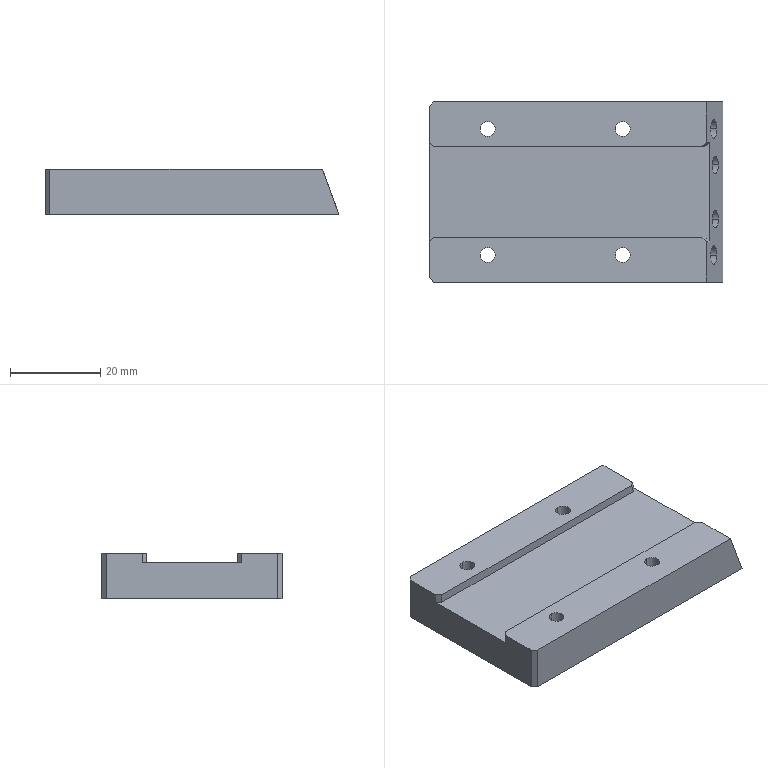Part | NX | 1 solid | 38 faces | box 65.2 x 40 x 10 mm | volume 22132 mm3 | plane 18 | cylinder 16 | cone 4 | commonest cylinder face diameters 3.3 x8 4 x4 4.2 x4
STEP:
#1=CARTESIAN_POINT('',(25.507,-6.,-5.132));
#2=VERTEX_POINT('',#1);
#3=CARTESIAN_POINT('',(26.875,-6.,-8.891));
#4=VERTEX_POINT('',#3);
#5=CARTESIAN_POINT('',(26.191,-6.,-7.012));
#6=DIRECTION('',(0.9397,0.,0.342));
#7=DIRECTION('',(0.342,0.,-0.9397));
#8=AXIS2_PLACEMENT_3D('',#5,#6,#7);
#9=CIRCLE('',#8,2.);
#10=EDGE_CURVE('',#2,#4,#9,.T.);
#11=ORIENTED_EDGE('',*,*,#10,.F.);
#12=CARTESIAN_POINT('',(30.206,-6.,-3.422));
#13=VERTEX_POINT('',#12);
#14=CARTESIAN_POINT('',(25.507,-6.,-5.132));
#15=DIRECTION('',(0.9397,0.,0.342));
#16=VECTOR('',#15,1000.);
#17=LINE('',#14,#16);
#18=EDGE_CURVE('',#2,#13,#17,.T.);
#19=ORIENTED_EDGE('',*,*,#18,.T.);
#20=CARTESIAN_POINT('',(31.574,-6.,-7.181));
#21=VERTEX_POINT('',#20);
#22=CARTESIAN_POINT('',(30.89,-6.,-5.302));
#23=DIRECTION('',(0.9397,0.,0.342));
#24=DIRECTION('',(0.342,0.,-0.9397));
#25=AXIS2_PLACEMENT_3D('',#22,#23,#24);
#26=CIRCLE('',#25,2.);
#27=EDGE_CURVE('',#13,#21,#26,.T.);
#28=ORIENTED_EDGE('',*,*,#27,.T.);
#29=CARTESIAN_POINT('',(26.875,-6.,-8.891));
#30=DIRECTION('',(0.9397,0.,0.342));
#31=VECTOR('',#30,1000.);
#32=LINE('',#29,#31);
#33=EDGE_CURVE('',#4,#21,#32,.T.);
#34=ORIENTED_EDGE('',*,*,#33,.F.);
#35=EDGE_LOOP('',(#11,#19,#28,#34));
#36=FACE_BOUND('',#35,.T.);
#37=CARTESIAN_POINT('',(26.191,-6.,-7.012));
#38=DIRECTION('',(0.9397,0.,0.342));
#39=DIRECTION('',(-0.342,0.,0.9397));
#40=AXIS2_PLACEMENT_3D('',#37,#38,#39);
#41=CYLINDRICAL_SURFACE('',#40,2.);
#42=ADVANCED_FACE('',(#36),#41,.F.);
#43=CARTESIAN_POINT('',(25.507,6.,-5.132));
#44=VERTEX_POINT('',#43);
#45=CARTESIAN_POINT('',(26.875,6.,-8.891));
#46=VERTEX_POINT('',#45);
#47=CARTESIAN_POINT('',(26.191,6.,-7.012));
#48=DIRECTION('',(0.9397,0.,0.342));
#49=DIRECTION('',(0.342,0.,-0.9397));
#50=AXIS2_PLACEMENT_3D('',#47,#48,#49);
#51=CIRCLE('',#50,2.);
#52=EDGE_CURVE('',#44,#46,#51,.T.);
#53=ORIENTED_EDGE('',*,*,#52,.F.);
#54=CARTESIAN_POINT('',(30.206,6.,-3.422));
#55=VERTEX_POINT('',#54);
#56=CARTESIAN_POINT('',(25.507,6.,-5.132));
#57=DIRECTION('',(0.9397,0.,0.342));
#58=VECTOR('',#57,1000.);
#59=LINE('',#56,#58);
#60=EDGE_CURVE('',#44,#55,#59,.T.);
#61=ORIENTED_EDGE('',*,*,#60,.T.);
#62=CARTESIAN_POINT('',(31.574,6.,-7.181));
#63=VERTEX_POINT('',#62);
#64=CARTESIAN_POINT('',(30.89,6.,-5.302));
#65=DIRECTION('',(0.9397,0.,0.342));
#66=DIRECTION('',(0.342,0.,-0.9397));
#67=AXIS2_PLACEMENT_3D('',#64,#65,#66);
#68=CIRCLE('',#67,2.);
#69=EDGE_CURVE('',#55,#63,#68,.T.);
#70=ORIENTED_EDGE('',*,*,#69,.T.);
#71=CARTESIAN_POINT('',(26.875,6.,-8.891));
#72=DIRECTION('',(0.9397,0.,0.342));
#73=VECTOR('',#72,1000.);
#74=LINE('',#71,#73);
#75=EDGE_CURVE('',#46,#63,#74,.T.);
#76=ORIENTED_EDGE('',*,*,#75,.F.);
#77=EDGE_LOOP('',(#53,#61,#70,#76));
#78=FACE_BOUND('',#77,.T.);
#79=CARTESIAN_POINT('',(26.191,6.,-7.012));
#80=DIRECTION('',(0.9397,0.,0.342));
#81=DIRECTION('',(-0.342,0.,0.9397));
#82=AXIS2_PLACEMENT_3D('',#79,#80,#81);
#83=CYLINDRICAL_SURFACE('',#82,2.);
#84=ADVANCED_FACE('',(#78),#83,.F.);
#85=CARTESIAN_POINT('',(21.372,-14.,-5.467));
#86=VERTEX_POINT('',#85);
#87=CARTESIAN_POINT('',(22.809,-14.,-9.413));
#88=VERTEX_POINT('',#87);
#89=CARTESIAN_POINT('',(22.091,-14.,-7.44));
#90=DIRECTION('',(0.9397,0.,0.342));
#91=DIRECTION('',(0.342,0.,-0.9397));
#92=AXIS2_PLACEMENT_3D('',#89,#90,#91);
#93=CIRCLE('',#92,2.1);
#94=EDGE_CURVE('',#86,#88,#93,.T.);
#95=ORIENTED_EDGE('',*,*,#94,.F.);
#96=CARTESIAN_POINT('',(29.83,-14.,-2.388));
#97=VERTEX_POINT('',#96);
#98=CARTESIAN_POINT('',(29.83,-14.,-2.388));
#99=DIRECTION('',(0.9397,0.,0.342));
#100=VECTOR('',#99,1000.);
#101=LINE('',#98,#100);
#102=EDGE_CURVE('',#86,#97,#101,.T.);
#103=ORIENTED_EDGE('',*,*,#102,.T.);
#104=CARTESIAN_POINT('',(31.266,-14.,-6.335));
#105=VERTEX_POINT('',#104);
#106=CARTESIAN_POINT('',(30.548,-14.,-4.362));
#107=DIRECTION('',(0.9397,0.,0.342));
#108=DIRECTION('',(0.342,0.,-0.9397));
#109=AXIS2_PLACEMENT_3D('',#106,#107,#108);
#110=CIRCLE('',#109,2.1);
#111=EDGE_CURVE('',#97,#105,#110,.T.);
#112=ORIENTED_EDGE('',*,*,#111,.T.);
#113=CARTESIAN_POINT('',(31.266,-14.,-6.335));
#114=DIRECTION('',(0.9397,0.,0.342));
#115=VECTOR('',#114,1000.);
#116=LINE('',#113,#115);
#117=EDGE_CURVE('',#88,#105,#116,.T.);
#118=ORIENTED_EDGE('',*,*,#117,.F.);
#119=EDGE_LOOP('',(#95,#103,#112,#118));
#120=FACE_BOUND('',#119,.T.);
#121=CARTESIAN_POINT('',(30.548,-14.,-4.362));
#122=DIRECTION('',(0.9397,0.,0.342));
#123=DIRECTION('',(-0.342,0.,0.9397));
#124=AXIS2_PLACEMENT_3D('',#121,#122,#123);
#125=CYLINDRICAL_SURFACE('',#124,2.1);
#126=ADVANCED_FACE('',(#120),#125,.F.);
#127=CARTESIAN_POINT('',(20.905,-14.,-7.872));
#128=VERTEX_POINT('',#127);
#129=CARTESIAN_POINT('',(22.809,-14.,-9.413));
#130=DIRECTION('',(0.7771,0.,-0.6293));
#131=VECTOR('',#130,1000.);
#132=LINE('',#129,#131);
#133=EDGE_CURVE('',#128,#88,#132,.T.);
#134=ORIENTED_EDGE('',*,*,#133,.F.);
#135=CARTESIAN_POINT('',(21.372,-14.,-5.467));
#136=DIRECTION('',(0.1908,0.,0.9816));
#137=VECTOR('',#136,1000.);
#138=LINE('',#135,#137);
#139=EDGE_CURVE('',#128,#86,#138,.T.);
#140=ORIENTED_EDGE('',*,*,#139,.T.);
#141=ORIENTED_EDGE('',*,*,#94,.T.);
#142=EDGE_LOOP('',(#134,#140,#141));
#143=FACE_BOUND('',#142,.T.);
#144=CARTESIAN_POINT('',(22.091,-14.,-7.44));
#145=DIRECTION('',(0.9397,0.,0.342));
#146=DIRECTION('',(-0.342,0.,0.9397));
#147=AXIS2_PLACEMENT_3D('',#144,#145,#146);
#148=CONICAL_SURFACE('',#147,2.1,1.03);
#149=ADVANCED_FACE('',(#143),#148,.F.);
#150=CARTESIAN_POINT('',(21.372,14.,-5.467));
#151=VERTEX_POINT('',#150);
#152=CARTESIAN_POINT('',(22.809,14.,-9.413));
#153=VERTEX_POINT('',#152);
#154=CARTESIAN_POINT('',(22.091,14.,-7.44));
#155=DIRECTION('',(0.9397,0.,0.342));
#156=DIRECTION('',(0.342,0.,-0.9397));
#157=AXIS2_PLACEMENT_3D('',#154,#155,#156);
#158=CIRCLE('',#157,2.1);
#159=EDGE_CURVE('',#151,#153,#158,.T.);
#160=ORIENTED_EDGE('',*,*,#159,.F.);
#161=CARTESIAN_POINT('',(29.83,14.,-2.388));
#162=VERTEX_POINT('',#161);
#163=CARTESIAN_POINT('',(29.83,14.,-2.388));
#164=DIRECTION('',(0.9397,0.,0.342));
#165=VECTOR('',#164,1000.);
#166=LINE('',#163,#165);
#167=EDGE_CURVE('',#151,#162,#166,.T.);
#168=ORIENTED_EDGE('',*,*,#167,.T.);
#169=CARTESIAN_POINT('',(31.266,14.,-6.335));
#170=VERTEX_POINT('',#169);
#171=CARTESIAN_POINT('',(30.548,14.,-4.362));
#172=DIRECTION('',(0.9397,0.,0.342));
#173=DIRECTION('',(0.342,0.,-0.9397));
#174=AXIS2_PLACEMENT_3D('',#171,#172,#173);
#175=CIRCLE('',#174,2.1);
#176=EDGE_CURVE('',#162,#170,#175,.T.);
#177=ORIENTED_EDGE('',*,*,#176,.T.);
#178=CARTESIAN_POINT('',(31.266,14.,-6.335));
#179=DIRECTION('',(0.9397,0.,0.342));
#180=VECTOR('',#179,1000.);
#181=LINE('',#178,#180);
#182=EDGE_CURVE('',#153,#170,#181,.T.);
#183=ORIENTED_EDGE('',*,*,#182,.F.);
#184=EDGE_LOOP('',(#160,#168,#177,#183));
#185=FACE_BOUND('',#184,.T.);
#186=CARTESIAN_POINT('',(30.548,14.,-4.362));
#187=DIRECTION('',(0.9397,0.,0.342));
#188=DIRECTION('',(-0.342,0.,0.9397));
#189=AXIS2_PLACEMENT_3D('',#186,#187,#188);
#190=CYLINDRICAL_SURFACE('',#189,2.1);
#191=ADVANCED_FACE('',(#185),#190,.F.);
#192=CARTESIAN_POINT('',(20.905,14.,-7.872));
#193=VERTEX_POINT('',#192);
#194=CARTESIAN_POINT('',(22.809,14.,-9.413));
#195=DIRECTION('',(0.7771,0.,-0.6293));
#196=VECTOR('',#195,1000.);
#197=LINE('',#194,#196);
#198=EDGE_CURVE('',#193,#153,#197,.T.);
#199=ORIENTED_EDGE('',*,*,#198,.F.);
#200=CARTESIAN_POINT('',(21.372,14.,-5.467));
#201=DIRECTION('',(0.1908,0.,0.9816));
#202=VECTOR('',#201,1000.);
#203=LINE('',#200,#202);
#204=EDGE_CURVE('',#193,#151,#203,.T.);
#205=ORIENTED_EDGE('',*,*,#204,.T.);
#206=ORIENTED_EDGE('',*,*,#159,.T.);
#207=EDGE_LOOP('',(#199,#205,#206));
#208=FACE_BOUND('',#207,.T.);
#209=CARTESIAN_POINT('',(22.091,14.,-7.44));
#210=DIRECTION('',(0.9397,0.,0.342));
#211=DIRECTION('',(-0.342,0.,0.9397));
#212=AXIS2_PLACEMENT_3D('',#209,#210,#211);
#213=CONICAL_SURFACE('',#212,2.1,1.03);
#214=ADVANCED_FACE('',(#208),#213,.F.);
#215=CARTESIAN_POINT('',(10.4,15.65,-10.));
#216=VERTEX_POINT('',#215);
#217=CARTESIAN_POINT('',(10.4,12.35,-10.));
#218=VERTEX_POINT('',#217);
#219=CARTESIAN_POINT('',(10.4,14.,-10.));
#220=DIRECTION('',(0.,0.,1.));
#221=DIRECTION('',(0.,-1.,0.));
#222=AXIS2_PLACEMENT_3D('',#219,#220,#221);
#223=CIRCLE('',#222,1.65);
#224=EDGE_CURVE('',#216,#218,#223,.T.);
#225=ORIENTED_EDGE('',*,*,#224,.F.);
#226=CARTESIAN_POINT('',(10.4,15.65,0.));
#227=VERTEX_POINT('',#226);
#228=CARTESIAN_POINT('',(10.4,15.65,0.));
#229=DIRECTION('',(0.,0.,1.));
#230=VECTOR('',#229,1000.);
#231=LINE('',#228,#230);
#232=EDGE_CURVE('',#216,#227,#231,.T.);
#233=ORIENTED_EDGE('',*,*,#232,.T.);
#234=CARTESIAN_POINT('',(10.4,12.35,0.));
#235=VERTEX_POINT('',#234);
#236=CARTESIAN_POINT('',(10.4,14.,0.));
#237=DIRECTION('',(0.,0.,1.));
#238=DIRECTION('',(0.,-1.,0.));
#239=AXIS2_PLACEMENT_3D('',#236,#237,#238);
#240=CIRCLE('',#239,1.65);
#241=EDGE_CURVE('',#227,#235,#240,.T.);
#242=ORIENTED_EDGE('',*,*,#241,.T.);
#243=CARTESIAN_POINT('',(10.4,12.35,0.));
#244=DIRECTION('',(0.,0.,1.));
#245=VECTOR('',#244,1000.);
#246=LINE('',#243,#245);
#247=EDGE_CURVE('',#218,#235,#246,.T.);
#248=ORIENTED_EDGE('',*,*,#247,.F.);
#249=EDGE_LOOP('',(#225,#233,#242,#248));
#250=FACE_BOUND('',#249,.T.);
#251=CARTESIAN_POINT('',(10.4,14.,0.));
#252=DIRECTION('',(0.,0.,1.));
#253=DIRECTION('',(0.,1.,0.));
#254=AXIS2_PLACEMENT_3D('',#251,#252,#253);
#255=CYLINDRICAL_SURFACE('',#254,1.65);
#256=ADVANCED_FACE('',(#250),#255,.F.);
#257=CARTESIAN_POINT('',(10.4,-12.35,-10.));
#258=VERTEX_POINT('',#257);
#259=CARTESIAN_POINT('',(10.4,-15.65,-10.));
#260=VERTEX_POINT('',#259);
#261=CARTESIAN_POINT('',(10.4,-14.,-10.));
#262=DIRECTION('',(0.,0.,1.));
#263=DIRECTION('',(0.,-1.,0.));
#264=AXIS2_PLACEMENT_3D('',#261,#262,#263);
#265=CIRCLE('',#264,1.65);
#266=EDGE_CURVE('',#258,#260,#265,.T.);
#267=ORIENTED_EDGE('',*,*,#266,.F.);
#268=CARTESIAN_POINT('',(10.4,-12.35,0.));
#269=VERTEX_POINT('',#268);
#270=CARTESIAN_POINT('',(10.4,-12.35,0.));
#271=DIRECTION('',(0.,0.,1.));
#272=VECTOR('',#271,1000.);
#273=LINE('',#270,#272);
#274=EDGE_CURVE('',#258,#269,#273,.T.);
#275=ORIENTED_EDGE('',*,*,#274,.T.);
#276=CARTESIAN_POINT('',(10.4,-15.65,0.));
#277=VERTEX_POINT('',#276);
#278=CARTESIAN_POINT('',(10.4,-14.,0.));
#279=DIRECTION('',(0.,0.,1.));
#280=DIRECTION('',(0.,-1.,0.));
#281=AXIS2_PLACEMENT_3D('',#278,#279,#280);
#282=CIRCLE('',#281,1.65);
#283=EDGE_CURVE('',#269,#277,#282,.T.);
#284=ORIENTED_EDGE('',*,*,#283,.T.);
#285=CARTESIAN_POINT('',(10.4,-15.65,0.));
#286=DIRECTION('',(0.,0.,1.));
#287=VECTOR('',#286,1000.);
#288=LINE('',#285,#287);
#289=EDGE_CURVE('',#260,#277,#288,.T.);
#290=ORIENTED_EDGE('',*,*,#289,.F.);
#291=EDGE_LOOP('',(#267,#275,#284,#290));
#292=FACE_BOUND('',#291,.T.);
#293=CARTESIAN_POINT('',(10.4,-14.,0.));
#294=DIRECTION('',(0.,0.,1.));
#295=DIRECTION('',(0.,1.,0.));
#296=AXIS2_PLACEMENT_3D('',#293,#294,#295);
#297=CYLINDRICAL_SURFACE('',#296,1.65);
#298=ADVANCED_FACE('',(#292),#297,.F.);
#299=CARTESIAN_POINT('',(-19.6,15.65,-10.));
#300=VERTEX_POINT('',#299);
#301=CARTESIAN_POINT('',(-19.6,12.35,-10.));
#302=VERTEX_POINT('',#301);
#303=CARTESIAN_POINT('',(-19.6,14.,-10.));
#304=DIRECTION('',(0.,0.,1.));
#305=DIRECTION('',(0.,-1.,0.));
#306=AXIS2_PLACEMENT_3D('',#303,#304,#305);
#307=CIRCLE('',#306,1.65);
#308=EDGE_CURVE('',#300,#302,#307,.T.);
#309=ORIENTED_EDGE('',*,*,#308,.F.);
#310=CARTESIAN_POINT('',(-19.6,15.65,0.));
#311=VERTEX_POINT('',#310);
#312=CARTESIAN_POINT('',(-19.6,15.65,0.));
#313=DIRECTION('',(0.,0.,1.));
#314=VECTOR('',#313,1000.);
#315=LINE('',#312,#314);
#316=EDGE_CURVE('',#300,#311,#315,.T.);
#317=ORIENTED_EDGE('',*,*,#316,.T.);
#318=CARTESIAN_POINT('',(-19.6,12.35,0.));
#319=VERTEX_POINT('',#318);
#320=CARTESIAN_POINT('',(-19.6,14.,0.));
#321=DIRECTION('',(0.,0.,1.));
#322=DIRECTION('',(0.,-1.,0.));
#323=AXIS2_PLACEMENT_3D('',#320,#321,#322);
#324=CIRCLE('',#323,1.65);
#325=EDGE_CURVE('',#311,#319,#324,.T.);
#326=ORIENTED_EDGE('',*,*,#325,.T.);
#327=CARTESIAN_POINT('',(-19.6,12.35,0.));
#328=DIRECTION('',(0.,0.,1.));
#329=VECTOR('',#328,1000.);
#330=LINE('',#327,#329);
#331=EDGE_CURVE('',#302,#319,#330,.T.);
#332=ORIENTED_EDGE('',*,*,#331,.F.);
#333=EDGE_LOOP('',(#309,#317,#326,#332));
#334=FACE_BOUND('',#333,.T.);
#335=CARTESIAN_POINT('',(-19.6,14.,0.));
#336=DIRECTION('',(0.,0.,1.));
#337=DIRECTION('',(0.,1.,0.));
#338=AXIS2_PLACEMENT_3D('',#335,#336,#337);
#339=CYLINDRICAL_SURFACE('',#338,1.65);
#340=ADVANCED_FACE('',(#334),#339,.F.);
#341=CARTESIAN_POINT('',(-19.6,-12.35,-10.));
#342=VERTEX_POINT('',#341);
#343=CARTESIAN_POINT('',(-19.6,-15.65,-10.));
#344=VERTEX_POINT('',#343);
#345=CARTESIAN_POINT('',(-19.6,-14.,-10.));
#346=DIRECTION('',(0.,0.,1.));
#347=DIRECTION('',(0.,-1.,0.));
#348=AXIS2_PLACEMENT_3D('',#345,#346,#347);
#349=CIRCLE('',#348,1.65);
#350=EDGE_CURVE('',#342,#344,#349,.T.);
#351=ORIENTED_EDGE('',*,*,#350,.F.);
#352=CARTESIAN_POINT('',(-19.6,-12.35,0.));
#353=VERTEX_POINT('',#352);
#354=CARTESIAN_POINT('',(-19.6,-12.35,0.));
#355=DIRECTION('',(0.,0.,1.));
#356=VECTOR('',#355,1000.);
#357=LINE('',#354,#356);
#358=EDGE_CURVE('',#342,#353,#357,.T.);
#359=ORIENTED_EDGE('',*,*,#358,.T.);
#360=CARTESIAN_POINT('',(-19.6,-15.65,0.));
#361=VERTEX_POINT('',#360);
#362=CARTESIAN_POINT('',(-19.6,-14.,0.));
#363=DIRECTION('',(0.,0.,1.));
#364=DIRECTION('',(0.,-1.,0.));
#365=AXIS2_PLACEMENT_3D('',#362,#363,#364);
#366=CIRCLE('',#365,1.65);
#367=EDGE_CURVE('',#353,#361,#366,.T.);
#368=ORIENTED_EDGE('',*,*,#367,.T.);
#369=CARTESIAN_POINT('',(-19.6,-15.65,0.));
#370=DIRECTION('',(0.,0.,1.));
#371=VECTOR('',#370,1000.);
#372=LINE('',#369,#371);
#373=EDGE_CURVE('',#344,#361,#372,.T.);
#374=ORIENTED_EDGE('',*,*,#373,.F.);
#375=EDGE_LOOP('',(#351,#359,#368,#374));
#376=FACE_BOUND('',#375,.T.);
#377=CARTESIAN_POINT('',(-19.6,-14.,0.));
#378=DIRECTION('',(0.,0.,1.));
#379=DIRECTION('',(0.,1.,0.));
#380=AXIS2_PLACEMENT_3D('',#377,#378,#379);
#381=CYLINDRICAL_SURFACE('',#380,1.65);
#382=ADVANCED_FACE('',(#376),#381,.F.);
#383=CARTESIAN_POINT('',(10.4,-14.,0.));
#384=DIRECTION('',(0.,0.,1.));
#385=DIRECTION('',(0.,-1.,0.));
#386=AXIS2_PLACEMENT_3D('',#383,#384,#385);
#387=CIRCLE('',#386,1.65);
#388=EDGE_CURVE('',#277,#269,#387,.T.);
#389=ORIENTED_EDGE('',*,*,#388,.F.);
#390=ORIENTED_EDGE('',*,*,#283,.F.);
#391=EDGE_LOOP('',(#389,#390));
#392=FACE_BOUND('',#391,.T.);
#393=CARTESIAN_POINT('',(-19.6,-14.,0.));
#394=DIRECTION('',(0.,0.,1.));
#395=DIRECTION('',(0.,-1.,0.));
#396=AXIS2_PLACEMENT_3D('',#393,#394,#395);
#397=CIRCLE('',#396,1.65);
#398=EDGE_CURVE('',#361,#353,#397,.T.);
#399=ORIENTED_EDGE('',*,*,#398,.F.);
#400=ORIENTED_EDGE('',*,*,#367,.F.);
#401=EDGE_LOOP('',(#399,#400));
#402=FACE_BOUND('',#401,.T.);
#403=CARTESIAN_POINT('',(-32.6,-19.,0.));
#404=VERTEX_POINT('',#403);
#405=CARTESIAN_POINT('',(-32.6,-11.,0.));
#406=VERTEX_POINT('',#405);
#407=CARTESIAN_POINT('',(-32.6,-20.,0.));
#408=DIRECTION('',(0.,1.,0.));
#409=VECTOR('',#408,1000.);
#410=LINE('',#407,#409);
#411=EDGE_CURVE('',#404,#406,#410,.T.);
#412=ORIENTED_EDGE('',*,*,#411,.F.);
#413=CARTESIAN_POINT('',(-31.6,-20.,0.));
#414=VERTEX_POINT('',#413);
#415=CARTESIAN_POINT('',(-32.6,-19.,0.));
#416=DIRECTION('',(0.7071,-0.7071,0.));
#417=VECTOR('',#416,1000.);
#418=LINE('',#415,#417);
#419=EDGE_CURVE('',#404,#414,#418,.T.);
#420=ORIENTED_EDGE('',*,*,#419,.T.);
#421=CARTESIAN_POINT('',(28.96,-20.,0.));
#422=VERTEX_POINT('',#421);
#423=CARTESIAN_POINT('',(32.6,-20.,0.));
#424=DIRECTION('',(-1.,0.,0.));
#425=VECTOR('',#424,1000.);
#426=LINE('',#423,#425);
#427=EDGE_CURVE('',#422,#414,#426,.T.);
#428=ORIENTED_EDGE('',*,*,#427,.F.);
#429=CARTESIAN_POINT('',(28.96,-11.,0.));
#430=VERTEX_POINT('',#429);
#431=CARTESIAN_POINT('',(28.96,-20.,0.));
#432=DIRECTION('',(0.,1.,0.));
#433=VECTOR('',#432,1000.);
#434=LINE('',#431,#433);
#435=EDGE_CURVE('',#422,#430,#434,.T.);
#436=ORIENTED_EDGE('',*,*,#435,.T.);
#437=CARTESIAN_POINT('',(27.896,-10.,0.));
#438=VERTEX_POINT('',#437);
#439=CARTESIAN_POINT('',(28.53,-10.595,0.));
#440=DIRECTION('',(-0.7287,0.6848,0.));
#441=VECTOR('',#440,1000.);
#442=LINE('',#439,#441);
#443=EDGE_CURVE('',#430,#438,#442,.T.);
#444=ORIENTED_EDGE('',*,*,#443,.T.);
#445=CARTESIAN_POINT('',(-31.6,-10.,0.));
#446=VERTEX_POINT('',#445);
#447=CARTESIAN_POINT('',(32.6,-10.,0.));
#448=DIRECTION('',(1.,0.,0.));
#449=VECTOR('',#448,1000.);
#450=LINE('',#447,#449);
#451=EDGE_CURVE('',#446,#438,#450,.T.);
#452=ORIENTED_EDGE('',*,*,#451,.F.);
#453=CARTESIAN_POINT('',(-31.6,-10.,0.));
#454=DIRECTION('',(-0.7071,-0.7071,0.));
#455=VECTOR('',#454,1000.);
#456=LINE('',#453,#455);
#457=EDGE_CURVE('',#446,#406,#456,.T.);
#458=ORIENTED_EDGE('',*,*,#457,.T.);
#459=EDGE_LOOP('',(#412,#420,#428,#436,#444,#452,#458));
#460=FACE_BOUND('',#459,.T.);
#461=CARTESIAN_POINT('',(0.,0.,0.));
#462=DIRECTION('',(0.,0.,-1.));
#463=DIRECTION('',(0.,-1.,0.));
#464=AXIS2_PLACEMENT_3D('',#461,#462,#463);
#465=PLANE('',#464);
#466=ADVANCED_FACE('',(#392,#402,#460),#465,.F.);
#467=CARTESIAN_POINT('',(-31.6,20.,-10.));
#468=VERTEX_POINT('',#467);
#469=CARTESIAN_POINT('',(32.6,20.,-10.));
#470=VERTEX_POINT('',#469);
#471=CARTESIAN_POINT('',(32.6,20.,-10.));
#472=DIRECTION('',(1.,0.,0.));
#473=VECTOR('',#472,1000.);
#474=LINE('',#471,#473);
#475=EDGE_CURVE('',#468,#470,#474,.T.);
#476=ORIENTED_EDGE('',*,*,#475,.F.);
#477=CARTESIAN_POINT('',(-31.6,20.,0.));
#478=VERTEX_POINT('',#477);
#479=CARTESIAN_POINT('',(-31.6,20.,-10.));
#480=DIRECTION('',(0.,0.,1.));
#481=VECTOR('',#480,1000.);
#482=LINE('',#479,#481);
#483=EDGE_CURVE('',#468,#478,#482,.T.);
#484=ORIENTED_EDGE('',*,*,#483,.T.);
#485=CARTESIAN_POINT('',(28.96,20.,0.));
#486=VERTEX_POINT('',#485);
#487=CARTESIAN_POINT('',(32.6,20.,0.));
#488=DIRECTION('',(1.,0.,0.));
#489=VECTOR('',#488,1000.);
#490=LINE('',#487,#489);
#491=EDGE_CURVE('',#478,#486,#490,.T.);
#492=ORIENTED_EDGE('',*,*,#491,.T.);
#493=CARTESIAN_POINT('',(28.96,20.,0.));
#494=DIRECTION('',(-0.342,0.,0.9397));
#495=VECTOR('',#494,1000.);
#496=LINE('',#493,#495);
#497=EDGE_CURVE('',#470,#486,#496,.T.);
#498=ORIENTED_EDGE('',*,*,#497,.F.);
#499=EDGE_LOOP('',(#476,#484,#492,#498));
#500=FACE_BOUND('',#499,.T.);
#501=CARTESIAN_POINT('',(32.6,20.,-10.));
#502=DIRECTION('',(0.,-1.,0.));
#503=DIRECTION('',(1.,0.,0.));
#504=AXIS2_PLACEMENT_3D('',#501,#502,#503);
#505=PLANE('',#504);
#506=ADVANCED_FACE('',(#500),#505,.F.);
#507=ORIENTED_EDGE('',*,*,#427,.T.);
#508=CARTESIAN_POINT('',(-31.6,-20.,-10.));
#509=VERTEX_POINT('',#508);
#510=CARTESIAN_POINT('',(-31.6,-20.,-10.));
#511=DIRECTION('',(0.,0.,-1.));
#512=VECTOR('',#511,1000.);
#513=LINE('',#510,#512);
#514=EDGE_CURVE('',#414,#509,#513,.T.);
#515=ORIENTED_EDGE('',*,*,#514,.T.);
#516=CARTESIAN_POINT('',(32.6,-20.,-10.));
#517=VERTEX_POINT('',#516);
#518=CARTESIAN_POINT('',(32.6,-20.,-10.));
#519=DIRECTION('',(-1.,0.,0.));
#520=VECTOR('',#519,1000.);
#521=LINE('',#518,#520);
#522=EDGE_CURVE('',#517,#509,#521,.T.);
#523=ORIENTED_EDGE('',*,*,#522,.F.);
#524=CARTESIAN_POINT('',(28.96,-20.,0.));
#525=DIRECTION('',(-0.342,0.,0.9397));
#526=VECTOR('',#525,1000.);
#527=LINE('',#524,#526);
#528=EDGE_CURVE('',#517,#422,#527,.T.);
#529=ORIENTED_EDGE('',*,*,#528,.T.);
#530=EDGE_LOOP('',(#507,#515,#523,#529));
#531=FACE_BOUND('',#530,.T.);
#532=CARTESIAN_POINT('',(32.6,-20.,-10.));
#533=DIRECTION('',(0.,1.,0.));
#534=DIRECTION('',(-1.,0.,0.));
#535=AXIS2_PLACEMENT_3D('',#532,#533,#534);
#536=PLANE('',#535);
#537=ADVANCED_FACE('',(#531),#536,.F.);
#538=CARTESIAN_POINT('',(-32.6,-19.,-10.));
#539=VERTEX_POINT('',#538);
#540=CARTESIAN_POINT('',(-32.6,19.,-10.));
#541=VERTEX_POINT('',#540);
#542=CARTESIAN_POINT('',(-32.6,-20.,-10.));
#543=DIRECTION('',(0.,1.,0.));
#544=VECTOR('',#543,1000.);
#545=LINE('',#542,#544);
#546=EDGE_CURVE('',#539,#541,#545,.T.);
#547=ORIENTED_EDGE('',*,*,#546,.F.);
#548=CARTESIAN_POINT('',(-32.6,-19.,-10.));
#549=DIRECTION('',(0.,0.,1.));
#550=VECTOR('',#549,1000.);
#551=LINE('',#548,#550);
#552=EDGE_CURVE('',#539,#404,#551,.T.);
#553=ORIENTED_EDGE('',*,*,#552,.T.);
#554=ORIENTED_EDGE('',*,*,#411,.T.);
#555=CARTESIAN_POINT('',(-32.6,-11.,-2.));
#556=VERTEX_POINT('',#555);
#557=CARTESIAN_POINT('',(-32.6,-11.,-10.));
#558=DIRECTION('',(0.,0.,-1.));
#559=VECTOR('',#558,1000.);
#560=LINE('',#557,#559);
#561=EDGE_CURVE('',#406,#556,#560,.T.);
#562=ORIENTED_EDGE('',*,*,#561,.T.);
#563=CARTESIAN_POINT('',(-32.6,11.,-2.));
#564=VERTEX_POINT('',#563);
#565=CARTESIAN_POINT('',(-32.6,10.,-2.));
#566=DIRECTION('',(0.,-1.,0.));
#567=VECTOR('',#566,1000.);
#568=LINE('',#565,#567);
#569=EDGE_CURVE('',#564,#556,#568,.T.);
#570=ORIENTED_EDGE('',*,*,#569,.F.);
#571=CARTESIAN_POINT('',(-32.6,11.,0.));
#572=VERTEX_POINT('',#571);
#573=CARTESIAN_POINT('',(-32.6,11.,-10.));
#574=DIRECTION('',(0.,0.,1.));
#575=VECTOR('',#574,1000.);
#576=LINE('',#573,#575);
#577=EDGE_CURVE('',#564,#572,#576,.T.);
#578=ORIENTED_EDGE('',*,*,#577,.T.);
#579=CARTESIAN_POINT('',(-32.6,19.,0.));
#580=VERTEX_POINT('',#579);
#581=CARTESIAN_POINT('',(-32.6,-20.,0.));
#582=DIRECTION('',(0.,1.,0.));
#583=VECTOR('',#582,1000.);
#584=LINE('',#581,#583);
#585=EDGE_CURVE('',#572,#580,#584,.T.);
#586=ORIENTED_EDGE('',*,*,#585,.T.);
#587=CARTESIAN_POINT('',(-32.6,19.,-10.));
#588=DIRECTION('',(0.,0.,-1.));
#589=VECTOR('',#588,1000.);
#590=LINE('',#587,#589);
#591=EDGE_CURVE('',#580,#541,#590,.T.);
#592=ORIENTED_EDGE('',*,*,#591,.T.);
#593=EDGE_LOOP('',(#547,#553,#554,#562,#570,#578,#586,#592));
#594=FACE_BOUND('',#593,.T.);
#595=CARTESIAN_POINT('',(-32.6,-20.,-10.));
#596=DIRECTION('',(1.,0.,0.));
#597=DIRECTION('',(0.,0.,1.));
#598=AXIS2_PLACEMENT_3D('',#595,#596,#597);
#599=PLANE('',#598);
#600=ADVANCED_FACE('',(#594),#599,.F.);
#601=CARTESIAN_POINT('',(10.4,14.,-10.));
#602=DIRECTION('',(0.,0.,1.));
#603=DIRECTION('',(0.,-1.,0.));
#604=AXIS2_PLACEMENT_3D('',#601,#602,#603);
#605=CIRCLE('',#604,1.65);
#606=EDGE_CURVE('',#218,#216,#605,.T.);
#607=ORIENTED_EDGE('',*,*,#606,.T.);
#608=ORIENTED_EDGE('',*,*,#224,.T.);
#609=EDGE_LOOP('',(#607,#608));
#610=FACE_BOUND('',#609,.T.);
#611=CARTESIAN_POINT('',(10.4,-14.,-10.));
#612=DIRECTION('',(0.,0.,1.));
#613=DIRECTION('',(0.,-1.,0.));
#614=AXIS2_PLACEMENT_3D('',#611,#612,#613);
#615=CIRCLE('',#614,1.65);
#616=EDGE_CURVE('',#260,#258,#615,.T.);
#617=ORIENTED_EDGE('',*,*,#616,.T.);
#618=ORIENTED_EDGE('',*,*,#266,.T.);
#619=EDGE_LOOP('',(#617,#618));
#620=FACE_BOUND('',#619,.T.);
#621=CARTESIAN_POINT('',(-19.6,14.,-10.));
#622=DIRECTION('',(0.,0.,1.));
#623=DIRECTION('',(0.,-1.,0.));
#624=AXIS2_PLACEMENT_3D('',#621,#622,#623);
#625=CIRCLE('',#624,1.65);
#626=EDGE_CURVE('',#302,#300,#625,.T.);
#627=ORIENTED_EDGE('',*,*,#626,.T.);
#628=ORIENTED_EDGE('',*,*,#308,.T.);
#629=EDGE_LOOP('',(#627,#628));
#630=FACE_BOUND('',#629,.T.);
#631=CARTESIAN_POINT('',(-19.6,-14.,-10.));
#632=DIRECTION('',(0.,0.,1.));
#633=DIRECTION('',(0.,-1.,0.));
#634=AXIS2_PLACEMENT_3D('',#631,#632,#633);
#635=CIRCLE('',#634,1.65);
#636=EDGE_CURVE('',#344,#342,#635,.T.);
#637=ORIENTED_EDGE('',*,*,#636,.T.);
#638=ORIENTED_EDGE('',*,*,#350,.T.);
#639=EDGE_LOOP('',(#637,#638));
#640=FACE_BOUND('',#639,.T.);
#641=ORIENTED_EDGE('',*,*,#522,.T.);
#642=CARTESIAN_POINT('',(-25.8,-25.8,-10.));
#643=DIRECTION('',(-0.7071,0.7071,0.));
#644=VECTOR('',#643,1000.);
#645=LINE('',#642,#644);
#646=EDGE_CURVE('',#509,#539,#645,.T.);
#647=ORIENTED_EDGE('',*,*,#646,.T.);
#648=ORIENTED_EDGE('',*,*,#546,.T.);
#649=CARTESIAN_POINT('',(-25.8,25.8,-10.));
#650=DIRECTION('',(0.7071,0.7071,0.));
#651=VECTOR('',#650,1000.);
#652=LINE('',#649,#651);
#653=EDGE_CURVE('',#541,#468,#652,.T.);
#654=ORIENTED_EDGE('',*,*,#653,.T.);
#655=ORIENTED_EDGE('',*,*,#475,.T.);
#656=CARTESIAN_POINT('',(32.6,-20.,-10.));
#657=DIRECTION('',(0.,-1.,0.));
#658=VECTOR('',#657,1000.);
#659=LINE('',#656,#658);
#660=EDGE_CURVE('',#470,#517,#659,.T.);
#661=ORIENTED_EDGE('',*,*,#660,.T.);
#662=EDGE_LOOP('',(#641,#647,#648,#654,#655,#661));
#663=FACE_BOUND('',#662,.T.);
#664=CARTESIAN_POINT('',(0.,0.,-10.));
#665=DIRECTION('',(0.,0.,-1.));
#666=DIRECTION('',(0.,-1.,0.));
#667=AXIS2_PLACEMENT_3D('',#664,#665,#666);
#668=PLANE('',#667);
#669=ADVANCED_FACE('',(#610,#620,#630,#640,#663),#668,.T.);
#670=CARTESIAN_POINT('',(10.4,14.,0.));
#671=DIRECTION('',(0.,0.,1.));
#672=DIRECTION('',(0.,-1.,0.));
#673=AXIS2_PLACEMENT_3D('',#670,#671,#672);
#674=CIRCLE('',#673,1.65);
#675=EDGE_CURVE('',#235,#227,#674,.T.);
#676=ORIENTED_EDGE('',*,*,#675,.F.);
#677=ORIENTED_EDGE('',*,*,#241,.F.);
#678=EDGE_LOOP('',(#676,#677));
#679=FACE_BOUND('',#678,.T.);
#680=CARTESIAN_POINT('',(-19.6,14.,0.));
#681=DIRECTION('',(0.,0.,1.));
#682=DIRECTION('',(0.,-1.,0.));
#683=AXIS2_PLACEMENT_3D('',#680,#681,#682);
#684=CIRCLE('',#683,1.65);
#685=EDGE_CURVE('',#319,#311,#684,.T.);
#686=ORIENTED_EDGE('',*,*,#685,.F.);
#687=ORIENTED_EDGE('',*,*,#325,.F.);
#688=EDGE_LOOP('',(#686,#687));
#689=FACE_BOUND('',#688,.T.);
#690=ORIENTED_EDGE('',*,*,#491,.F.);
#691=CARTESIAN_POINT('',(-31.6,20.,0.));
#692=DIRECTION('',(-0.7071,-0.7071,0.));
#693=VECTOR('',#692,1000.);
#694=LINE('',#691,#693);
#695=EDGE_CURVE('',#478,#580,#694,.T.);
#696=ORIENTED_EDGE('',*,*,#695,.T.);
#697=ORIENTED_EDGE('',*,*,#585,.F.);
#698=CARTESIAN_POINT('',(-31.6,10.,0.));
#699=VERTEX_POINT('',#698);
#700=CARTESIAN_POINT('',(-32.6,11.,0.));
#701=DIRECTION('',(0.7071,-0.7071,0.));
#702=VECTOR('',#701,1000.);
#703=LINE('',#700,#702);
#704=EDGE_CURVE('',#572,#699,#703,.T.);
#705=ORIENTED_EDGE('',*,*,#704,.T.);
#706=CARTESIAN_POINT('',(27.896,10.,0.));
#707=VERTEX_POINT('',#706);
#708=CARTESIAN_POINT('',(32.6,10.,0.));
#709=DIRECTION('',(-1.,0.,0.));
#710=VECTOR('',#709,1000.);
#711=LINE('',#708,#710);
#712=EDGE_CURVE('',#707,#699,#711,.T.);
#713=ORIENTED_EDGE('',*,*,#712,.F.);
#714=CARTESIAN_POINT('',(28.96,11.,0.));
#715=VERTEX_POINT('',#714);
#716=CARTESIAN_POINT('',(28.53,10.595,0.));
#717=DIRECTION('',(0.7287,0.6848,0.));
#718=VECTOR('',#717,1000.);
#719=LINE('',#716,#718);
#720=EDGE_CURVE('',#707,#715,#719,.T.);
#721=ORIENTED_EDGE('',*,*,#720,.T.);
#722=CARTESIAN_POINT('',(28.96,-20.,0.));
#723=DIRECTION('',(0.,1.,0.));
#724=VECTOR('',#723,1000.);
#725=LINE('',#722,#724);
#726=EDGE_CURVE('',#715,#486,#725,.T.);
#727=ORIENTED_EDGE('',*,*,#726,.T.);
#728=EDGE_LOOP('',(#690,#696,#697,#705,#713,#721,#727));
#729=FACE_BOUND('',#728,.T.);
#730=CARTESIAN_POINT('',(0.,0.,0.));
#731=DIRECTION('',(0.,0.,-1.));
#732=DIRECTION('',(0.,-1.,0.));
#733=AXIS2_PLACEMENT_3D('',#730,#731,#732);
#734=PLANE('',#733);
#735=ADVANCED_FACE('',(#679,#689,#729),#734,.F.);
#736=CARTESIAN_POINT('',(-31.6,-10.,-2.));
#737=VERTEX_POINT('',#736);
#738=CARTESIAN_POINT('',(28.624,-10.,-2.));
#739=VERTEX_POINT('',#738);
#740=CARTESIAN_POINT('',(32.6,-10.,-2.));
#741=DIRECTION('',(1.,0.,0.));
#742=VECTOR('',#741,1000.);
#743=LINE('',#740,#742);
#744=EDGE_CURVE('',#737,#739,#743,.T.);
#745=ORIENTED_EDGE('',*,*,#744,.F.);
#746=CARTESIAN_POINT('',(-31.6,-10.,-2.));
#747=DIRECTION('',(0.,0.,1.));
#748=VECTOR('',#747,1000.);
#749=LINE('',#746,#748);
#750=EDGE_CURVE('',#737,#446,#749,.T.);
#751=ORIENTED_EDGE('',*,*,#750,.T.);
#752=ORIENTED_EDGE('',*,*,#451,.T.);
#753=CARTESIAN_POINT('',(29.089,-10.,-3.278));
#754=DIRECTION('',(0.342,0.,-0.9397));
#755=VECTOR('',#754,1000.);
#756=LINE('',#753,#755);
#757=EDGE_CURVE('',#438,#739,#756,.T.);
#758=ORIENTED_EDGE('',*,*,#757,.T.);
#759=EDGE_LOOP('',(#745,#751,#752,#758));
#760=FACE_BOUND('',#759,.T.);
#761=CARTESIAN_POINT('',(32.6,-10.,-2.));
#762=DIRECTION('',(0.,-1.,0.));
#763=DIRECTION('',(0.,0.,1.));
#764=AXIS2_PLACEMENT_3D('',#761,#762,#763);
#765=PLANE('',#764);
#766=ADVANCED_FACE('',(#760),#765,.F.);
#767=ORIENTED_EDGE('',*,*,#712,.T.);
#768=CARTESIAN_POINT('',(-31.6,10.,-2.));
#769=VERTEX_POINT('',#768);
#770=CARTESIAN_POINT('',(-31.6,10.,-2.));
#771=DIRECTION('',(0.,0.,-1.));
#772=VECTOR('',#771,1000.);
#773=LINE('',#770,#772);
#774=EDGE_CURVE('',#699,#769,#773,.T.);
#775=ORIENTED_EDGE('',*,*,#774,.T.);
#776=CARTESIAN_POINT('',(28.624,10.,-2.));
#777=VERTEX_POINT('',#776);
#778=CARTESIAN_POINT('',(32.6,10.,-2.));
#779=DIRECTION('',(-1.,0.,0.));
#780=VECTOR('',#779,1000.);
#781=LINE('',#778,#780);
#782=EDGE_CURVE('',#777,#769,#781,.T.);
#783=ORIENTED_EDGE('',*,*,#782,.F.);
#784=CARTESIAN_POINT('',(29.089,10.,-3.278));
#785=DIRECTION('',(-0.342,0.,0.9397));
#786=VECTOR('',#785,1000.);
#787=LINE('',#784,#786);
#788=EDGE_CURVE('',#777,#707,#787,.T.);
#789=ORIENTED_EDGE('',*,*,#788,.T.);
#790=EDGE_LOOP('',(#767,#775,#783,#789));
#791=FACE_BOUND('',#790,.T.);
#792=CARTESIAN_POINT('',(32.6,10.,-2.));
#793=DIRECTION('',(0.,1.,0.));
#794=DIRECTION('',(0.,0.,-1.));
#795=AXIS2_PLACEMENT_3D('',#792,#793,#794);
#796=PLANE('',#795);
#797=ADVANCED_FACE('',(#791),#796,.F.);
#798=CARTESIAN_POINT('',(29.688,11.,-2.));
#799=VERTEX_POINT('',#798);
#800=CARTESIAN_POINT('',(29.688,-11.,-2.));
#801=VERTEX_POINT('',#800);
#802=CARTESIAN_POINT('',(29.688,0.,-2.));
#803=DIRECTION('',(0.,-1.,0.));
#804=VECTOR('',#803,1000.);
#805=LINE('',#802,#804);
#806=EDGE_CURVE('',#799,#801,#805,.T.);
#807=ORIENTED_EDGE('',*,*,#806,.F.);
#808=CARTESIAN_POINT('',(28.871,10.232,-2.));
#809=DIRECTION('',(-0.7287,-0.6848,0.));
#810=VECTOR('',#809,1000.);
#811=LINE('',#808,#810);
#812=EDGE_CURVE('',#799,#777,#811,.T.);
#813=ORIENTED_EDGE('',*,*,#812,.T.);
#814=ORIENTED_EDGE('',*,*,#782,.T.);
#815=CARTESIAN_POINT('',(-32.6,11.,-2.));
#816=DIRECTION('',(-0.7071,0.7071,0.));
#817=VECTOR('',#816,1000.);
#818=LINE('',#815,#817);
#819=EDGE_CURVE('',#769,#564,#818,.T.);
#820=ORIENTED_EDGE('',*,*,#819,.T.);
#821=ORIENTED_EDGE('',*,*,#569,.T.);
#822=CARTESIAN_POINT('',(-31.6,-10.,-2.));
#823=DIRECTION('',(0.7071,0.7071,0.));
#824=VECTOR('',#823,1000.);
#825=LINE('',#822,#824);
#826=EDGE_CURVE('',#556,#737,#825,.T.);
#827=ORIENTED_EDGE('',*,*,#826,.T.);
#828=ORIENTED_EDGE('',*,*,#744,.T.);
#829=CARTESIAN_POINT('',(28.871,-10.232,-2.));
#830=DIRECTION('',(0.7287,-0.6848,0.));
#831=VECTOR('',#830,1000.);
#832=LINE('',#829,#831);
#833=EDGE_CURVE('',#739,#801,#832,.T.);
#834=ORIENTED_EDGE('',*,*,#833,.T.);
#835=EDGE_LOOP('',(#807,#813,#814,#820,#821,#827,#828,#834));
#836=FACE_BOUND('',#835,.T.);
#837=CARTESIAN_POINT('',(0.,0.,-2.));
#838=DIRECTION('',(0.,0.,1.));
#839=DIRECTION('',(0.,1.,0.));
#840=AXIS2_PLACEMENT_3D('',#837,#838,#839);
#841=PLANE('',#840);
#842=ADVANCED_FACE('',(#836),#841,.T.);
#843=ORIENTED_EDGE('',*,*,#358,.F.);
#844=ORIENTED_EDGE('',*,*,#636,.F.);
#845=ORIENTED_EDGE('',*,*,#373,.T.);
#846=ORIENTED_EDGE('',*,*,#398,.T.);
#847=EDGE_LOOP('',(#843,#844,#845,#846));
#848=FACE_BOUND('',#847,.T.);
#849=CARTESIAN_POINT('',(-19.6,-14.,0.));
#850=DIRECTION('',(0.,0.,1.));
#851=DIRECTION('',(0.,1.,0.));
#852=AXIS2_PLACEMENT_3D('',#849,#850,#851);
#853=CYLINDRICAL_SURFACE('',#852,1.65);
#854=ADVANCED_FACE('',(#848),#853,.F.);
#855=ORIENTED_EDGE('',*,*,#316,.F.);
#856=ORIENTED_EDGE('',*,*,#626,.F.);
#857=ORIENTED_EDGE('',*,*,#331,.T.);
#858=ORIENTED_EDGE('',*,*,#685,.T.);
#859=EDGE_LOOP('',(#855,#856,#857,#858));
#860=FACE_BOUND('',#859,.T.);
#861=CARTESIAN_POINT('',(-19.6,14.,0.));
#862=DIRECTION('',(0.,0.,1.));
#863=DIRECTION('',(0.,1.,0.));
#864=AXIS2_PLACEMENT_3D('',#861,#862,#863);
#865=CYLINDRICAL_SURFACE('',#864,1.65);
#866=ADVANCED_FACE('',(#860),#865,.F.);
#867=ORIENTED_EDGE('',*,*,#274,.F.);
#868=ORIENTED_EDGE('',*,*,#616,.F.);
#869=ORIENTED_EDGE('',*,*,#289,.T.);
#870=ORIENTED_EDGE('',*,*,#388,.T.);
#871=EDGE_LOOP('',(#867,#868,#869,#870));
#872=FACE_BOUND('',#871,.T.);
#873=CARTESIAN_POINT('',(10.4,-14.,0.));
#874=DIRECTION('',(0.,0.,1.));
#875=DIRECTION('',(0.,1.,0.));
#876=AXIS2_PLACEMENT_3D('',#873,#874,#875);
#877=CYLINDRICAL_SURFACE('',#876,1.65);
#878=ADVANCED_FACE('',(#872),#877,.F.);
#879=ORIENTED_EDGE('',*,*,#232,.F.);
#880=ORIENTED_EDGE('',*,*,#606,.F.);
#881=ORIENTED_EDGE('',*,*,#247,.T.);
#882=ORIENTED_EDGE('',*,*,#675,.T.);
#883=EDGE_LOOP('',(#879,#880,#881,#882));
#884=FACE_BOUND('',#883,.T.);
#885=CARTESIAN_POINT('',(10.4,14.,0.));
#886=DIRECTION('',(0.,0.,1.));
#887=DIRECTION('',(0.,1.,0.));
#888=AXIS2_PLACEMENT_3D('',#885,#886,#887);
#889=CYLINDRICAL_SURFACE('',#888,1.65);
#890=ADVANCED_FACE('',(#884),#889,.F.);
#891=CARTESIAN_POINT('',(30.89,-6.,-5.302));
#892=DIRECTION('',(0.9397,0.,0.342));
#893=DIRECTION('',(0.342,0.,-0.9397));
#894=AXIS2_PLACEMENT_3D('',#891,#892,#893);
#895=CIRCLE('',#894,2.);
#896=EDGE_CURVE('',#21,#13,#895,.T.);
#897=ORIENTED_EDGE('',*,*,#896,.F.);
#898=ORIENTED_EDGE('',*,*,#27,.F.);
#899=EDGE_LOOP('',(#897,#898));
#900=FACE_BOUND('',#899,.T.);
#901=CARTESIAN_POINT('',(30.89,6.,-5.302));
#902=DIRECTION('',(0.9397,0.,0.342));
#903=DIRECTION('',(0.342,0.,-0.9397));
#904=AXIS2_PLACEMENT_3D('',#901,#902,#903);
#905=CIRCLE('',#904,2.);
#906=EDGE_CURVE('',#63,#55,#905,.T.);
#907=ORIENTED_EDGE('',*,*,#906,.F.);
#908=ORIENTED_EDGE('',*,*,#69,.F.);
#909=EDGE_LOOP('',(#907,#908));
#910=FACE_BOUND('',#909,.T.);
#911=CARTESIAN_POINT('',(30.548,-14.,-4.362));
#912=DIRECTION('',(0.9397,0.,0.342));
#913=DIRECTION('',(0.342,0.,-0.9397));
#914=AXIS2_PLACEMENT_3D('',#911,#912,#913);
#915=CIRCLE('',#914,2.1);
#916=EDGE_CURVE('',#105,#97,#915,.T.);
#917=ORIENTED_EDGE('',*,*,#916,.F.);
#918=ORIENTED_EDGE('',*,*,#111,.F.);
#919=EDGE_LOOP('',(#917,#918));
#920=FACE_BOUND('',#919,.T.);
#921=CARTESIAN_POINT('',(30.548,14.,-4.362));
#922=DIRECTION('',(0.9397,0.,0.342));
#923=DIRECTION('',(0.342,0.,-0.9397));
#924=AXIS2_PLACEMENT_3D('',#921,#922,#923);
#925=CIRCLE('',#924,2.1);
#926=EDGE_CURVE('',#170,#162,#925,.T.);
#927=ORIENTED_EDGE('',*,*,#926,.F.);
#928=ORIENTED_EDGE('',*,*,#176,.F.);
#929=EDGE_LOOP('',(#927,#928));
#930=FACE_BOUND('',#929,.T.);
#931=ORIENTED_EDGE('',*,*,#806,.T.);
#932=CARTESIAN_POINT('',(28.96,-11.,0.));
#933=DIRECTION('',(-0.342,0.,0.9397));
#934=VECTOR('',#933,1000.);
#935=LINE('',#932,#934);
#936=EDGE_CURVE('',#801,#430,#935,.T.);
#937=ORIENTED_EDGE('',*,*,#936,.T.);
#938=ORIENTED_EDGE('',*,*,#435,.F.);
#939=ORIENTED_EDGE('',*,*,#528,.F.);
#940=ORIENTED_EDGE('',*,*,#660,.F.);
#941=ORIENTED_EDGE('',*,*,#497,.T.);
#942=ORIENTED_EDGE('',*,*,#726,.F.);
#943=CARTESIAN_POINT('',(28.96,11.,0.));
#944=DIRECTION('',(0.342,0.,-0.9397));
#945=VECTOR('',#944,1000.);
#946=LINE('',#943,#945);
#947=EDGE_CURVE('',#715,#799,#946,.T.);
#948=ORIENTED_EDGE('',*,*,#947,.T.);
#949=EDGE_LOOP('',(#931,#937,#938,#939,#940,#941,#942,#948));
#950=FACE_BOUND('',#949,.T.);
#951=CARTESIAN_POINT('',(28.96,-20.,0.));
#952=DIRECTION('',(-0.9397,0.,-0.342));
#953=DIRECTION('',(0.342,0.,-0.9397));
#954=AXIS2_PLACEMENT_3D('',#951,#952,#953);
#955=PLANE('',#954);
#956=ADVANCED_FACE('',(#900,#910,#920,#930,#950),#955,.F.);
#957=ORIENTED_EDGE('',*,*,#204,.F.);
#958=ORIENTED_EDGE('',*,*,#198,.T.);
#959=CARTESIAN_POINT('',(22.091,14.,-7.44));
#960=DIRECTION('',(0.9397,0.,0.342));
#961=DIRECTION('',(0.342,0.,-0.9397));
#962=AXIS2_PLACEMENT_3D('',#959,#960,#961);
#963=CIRCLE('',#962,2.1);
#964=EDGE_CURVE('',#153,#151,#963,.T.);
#965=ORIENTED_EDGE('',*,*,#964,.T.);
#966=EDGE_LOOP('',(#957,#958,#965));
#967=FACE_BOUND('',#966,.T.);
#968=CARTESIAN_POINT('',(22.091,14.,-7.44));
#969=DIRECTION('',(0.9397,0.,0.342));
#970=DIRECTION('',(-0.342,0.,0.9397));
#971=AXIS2_PLACEMENT_3D('',#968,#969,#970);
#972=CONICAL_SURFACE('',#971,2.1,1.03);
#973=ADVANCED_FACE('',(#967),#972,.F.);
#974=ORIENTED_EDGE('',*,*,#167,.F.);
#975=ORIENTED_EDGE('',*,*,#964,.F.);
#976=ORIENTED_EDGE('',*,*,#182,.T.);
#977=ORIENTED_EDGE('',*,*,#926,.T.);
#978=EDGE_LOOP('',(#974,#975,#976,#977));
#979=FACE_BOUND('',#978,.T.);
#980=CARTESIAN_POINT('',(30.548,14.,-4.362));
#981=DIRECTION('',(0.9397,0.,0.342));
#982=DIRECTION('',(-0.342,0.,0.9397));
#983=AXIS2_PLACEMENT_3D('',#980,#981,#982);
#984=CYLINDRICAL_SURFACE('',#983,2.1);
#985=ADVANCED_FACE('',(#979),#984,.F.);
#986=ORIENTED_EDGE('',*,*,#139,.F.);
#987=ORIENTED_EDGE('',*,*,#133,.T.);
#988=CARTESIAN_POINT('',(22.091,-14.,-7.44));
#989=DIRECTION('',(0.9397,0.,0.342));
#990=DIRECTION('',(0.342,0.,-0.9397));
#991=AXIS2_PLACEMENT_3D('',#988,#989,#990);
#992=CIRCLE('',#991,2.1);
#993=EDGE_CURVE('',#88,#86,#992,.T.);
#994=ORIENTED_EDGE('',*,*,#993,.T.);
#995=EDGE_LOOP('',(#986,#987,#994));
#996=FACE_BOUND('',#995,.T.);
#997=CARTESIAN_POINT('',(22.091,-14.,-7.44));
#998=DIRECTION('',(0.9397,0.,0.342));
#999=DIRECTION('',(-0.342,0.,0.9397));
#1000=AXIS2_PLACEMENT_3D('',#997,#998,#999);
#1001=CONICAL_SURFACE('',#1000,2.1,1.03);
#1002=ADVANCED_FACE('',(#996),#1001,.F.);
#1003=ORIENTED_EDGE('',*,*,#102,.F.);
#1004=ORIENTED_EDGE('',*,*,#993,.F.);
#1005=ORIENTED_EDGE('',*,*,#117,.T.);
#1006=ORIENTED_EDGE('',*,*,#916,.T.);
#1007=EDGE_LOOP('',(#1003,#1004,#1005,#1006));
#1008=FACE_BOUND('',#1007,.T.);
#1009=CARTESIAN_POINT('',(30.548,-14.,-4.362));
#1010=DIRECTION('',(0.9397,0.,0.342));
#1011=DIRECTION('',(-0.342,0.,0.9397));
#1012=AXIS2_PLACEMENT_3D('',#1009,#1010,#1011);
#1013=CYLINDRICAL_SURFACE('',#1012,2.1);
#1014=ADVANCED_FACE('',(#1008),#1013,.F.);
#1015=ORIENTED_EDGE('',*,*,#60,.F.);
#1016=CARTESIAN_POINT('',(26.191,6.,-7.012));
#1017=DIRECTION('',(0.9397,0.,0.342));
#1018=DIRECTION('',(0.342,0.,-0.9397));
#1019=AXIS2_PLACEMENT_3D('',#1016,#1017,#1018);
#1020=CIRCLE('',#1019,2.);
#1021=EDGE_CURVE('',#46,#44,#1020,.T.);
#1022=ORIENTED_EDGE('',*,*,#1021,.F.);
#1023=ORIENTED_EDGE('',*,*,#75,.T.);
#1024=ORIENTED_EDGE('',*,*,#906,.T.);
#1025=EDGE_LOOP('',(#1015,#1022,#1023,#1024));
#1026=FACE_BOUND('',#1025,.T.);
#1027=CARTESIAN_POINT('',(26.191,6.,-7.012));
#1028=DIRECTION('',(0.9397,0.,0.342));
#1029=DIRECTION('',(-0.342,0.,0.9397));
#1030=AXIS2_PLACEMENT_3D('',#1027,#1028,#1029);
#1031=CYLINDRICAL_SURFACE('',#1030,2.);
#1032=ADVANCED_FACE('',(#1026),#1031,.F.);
#1033=ORIENTED_EDGE('',*,*,#1021,.T.);
#1034=ORIENTED_EDGE('',*,*,#52,.T.);
#1035=EDGE_LOOP('',(#1033,#1034));
#1036=FACE_BOUND('',#1035,.T.);
#1037=CARTESIAN_POINT('',(26.191,6.,-7.012));
#1038=DIRECTION('',(0.9397,0.,0.342));
#1039=DIRECTION('',(-0.342,0.,0.9397));
#1040=AXIS2_PLACEMENT_3D('',#1037,#1038,#1039);
#1041=PLANE('',#1040);
#1042=ADVANCED_FACE('',(#1036),#1041,.T.);
#1043=ORIENTED_EDGE('',*,*,#18,.F.);
#1044=CARTESIAN_POINT('',(26.191,-6.,-7.012));
#1045=DIRECTION('',(0.9397,0.,0.342));
#1046=DIRECTION('',(0.342,0.,-0.9397));
#1047=AXIS2_PLACEMENT_3D('',#1044,#1045,#1046);
#1048=CIRCLE('',#1047,2.);
#1049=EDGE_CURVE('',#4,#2,#1048,.T.);
#1050=ORIENTED_EDGE('',*,*,#1049,.F.);
#1051=ORIENTED_EDGE('',*,*,#33,.T.);
#1052=ORIENTED_EDGE('',*,*,#896,.T.);
#1053=EDGE_LOOP('',(#1043,#1050,#1051,#1052));
#1054=FACE_BOUND('',#1053,.T.);
#1055=CARTESIAN_POINT('',(26.191,-6.,-7.012));
#1056=DIRECTION('',(0.9397,0.,0.342));
#1057=DIRECTION('',(-0.342,0.,0.9397));
#1058=AXIS2_PLACEMENT_3D('',#1055,#1056,#1057);
#1059=CYLINDRICAL_SURFACE('',#1058,2.);
#1060=ADVANCED_FACE('',(#1054),#1059,.F.);
#1061=ORIENTED_EDGE('',*,*,#1049,.T.);
#1062=ORIENTED_EDGE('',*,*,#10,.T.);
#1063=EDGE_LOOP('',(#1061,#1062));
#1064=FACE_BOUND('',#1063,.T.);
#1065=CARTESIAN_POINT('',(26.191,-6.,-7.012));
#1066=DIRECTION('',(0.9397,0.,0.342));
#1067=DIRECTION('',(-0.342,0.,0.9397));
#1068=AXIS2_PLACEMENT_3D('',#1065,#1066,#1067);
#1069=PLANE('',#1068);
#1070=ADVANCED_FACE('',(#1064),#1069,.T.);
#1071=ORIENTED_EDGE('',*,*,#646,.F.);
#1072=ORIENTED_EDGE('',*,*,#514,.F.);
#1073=ORIENTED_EDGE('',*,*,#419,.F.);
#1074=ORIENTED_EDGE('',*,*,#552,.F.);
#1075=EDGE_LOOP('',(#1071,#1072,#1073,#1074));
#1076=FACE_BOUND('',#1075,.T.);
#1077=CARTESIAN_POINT('',(-32.6,-19.,-10.));
#1078=DIRECTION('',(0.7071,0.7071,0.));
#1079=DIRECTION('',(0.,0.,-1.));
#1080=AXIS2_PLACEMENT_3D('',#1077,#1078,#1079);
#1081=PLANE('',#1080);
#1082=ADVANCED_FACE('',(#1076),#1081,.F.);
#1083=ORIENTED_EDGE('',*,*,#653,.F.);
#1084=ORIENTED_EDGE('',*,*,#591,.F.);
#1085=ORIENTED_EDGE('',*,*,#695,.F.);
#1086=ORIENTED_EDGE('',*,*,#483,.F.);
#1087=EDGE_LOOP('',(#1083,#1084,#1085,#1086));
#1088=FACE_BOUND('',#1087,.T.);
#1089=CARTESIAN_POINT('',(-31.6,20.,-10.));
#1090=DIRECTION('',(0.7071,-0.7071,0.));
#1091=DIRECTION('',(0.,0.,-1.));
#1092=AXIS2_PLACEMENT_3D('',#1089,#1090,#1091);
#1093=PLANE('',#1092);
#1094=ADVANCED_FACE('',(#1088),#1093,.F.);
#1095=ORIENTED_EDGE('',*,*,#826,.F.);
#1096=ORIENTED_EDGE('',*,*,#561,.F.);
#1097=ORIENTED_EDGE('',*,*,#457,.F.);
#1098=ORIENTED_EDGE('',*,*,#750,.F.);
#1099=EDGE_LOOP('',(#1095,#1096,#1097,#1098));
#1100=FACE_BOUND('',#1099,.T.);
#1101=CARTESIAN_POINT('',(-31.6,-10.,-2.));
#1102=DIRECTION('',(0.7071,-0.7071,0.));
#1103=DIRECTION('',(0.,0.,-1.));
#1104=AXIS2_PLACEMENT_3D('',#1101,#1102,#1103);
#1105=PLANE('',#1104);
#1106=ADVANCED_FACE('',(#1100),#1105,.F.);
#1107=ORIENTED_EDGE('',*,*,#819,.F.);
#1108=ORIENTED_EDGE('',*,*,#774,.F.);
#1109=ORIENTED_EDGE('',*,*,#704,.F.);
#1110=ORIENTED_EDGE('',*,*,#577,.F.);
#1111=EDGE_LOOP('',(#1107,#1108,#1109,#1110));
#1112=FACE_BOUND('',#1111,.T.);
#1113=CARTESIAN_POINT('',(-32.6,11.,-10.));
#1114=DIRECTION('',(0.7071,0.7071,0.));
#1115=DIRECTION('',(0.,0.,-1.));
#1116=AXIS2_PLACEMENT_3D('',#1113,#1114,#1115);
#1117=PLANE('',#1116);
#1118=ADVANCED_FACE('',(#1112),#1117,.F.);
#1119=ORIENTED_EDGE('',*,*,#443,.F.);
#1120=ORIENTED_EDGE('',*,*,#936,.F.);
#1121=ORIENTED_EDGE('',*,*,#833,.F.);
#1122=ORIENTED_EDGE('',*,*,#757,.F.);
#1123=EDGE_LOOP('',(#1119,#1120,#1121,#1122));
#1124=FACE_BOUND('',#1123,.T.);
#1125=CARTESIAN_POINT('',(29.089,-10.,-3.278));
#1126=DIRECTION('',(-0.6645,-0.7071,-0.2418));
#1127=DIRECTION('',(-0.342,0.,0.9397));
#1128=AXIS2_PLACEMENT_3D('',#1125,#1126,#1127);
#1129=PLANE('',#1128);
#1130=ADVANCED_FACE('',(#1124),#1129,.F.);
#1131=ORIENTED_EDGE('',*,*,#812,.F.);
#1132=ORIENTED_EDGE('',*,*,#947,.F.);
#1133=ORIENTED_EDGE('',*,*,#720,.F.);
#1134=ORIENTED_EDGE('',*,*,#788,.F.);
#1135=EDGE_LOOP('',(#1131,#1132,#1133,#1134));
#1136=FACE_BOUND('',#1135,.T.);
#1137=CARTESIAN_POINT('',(29.089,10.,-3.278));
#1138=DIRECTION('',(-0.6645,0.7071,-0.2418));
#1139=DIRECTION('',(0.342,0.,-0.9397));
#1140=AXIS2_PLACEMENT_3D('',#1137,#1138,#1139);
#1141=PLANE('',#1140);
#1142=ADVANCED_FACE('',(#1136),#1141,.F.);
#1143=CLOSED_SHELL('',(#42,#84,#126,#149,#191,#214,#256,#298,#340,#382,#466,#506,#537,#600,#669,#735,#766,#797,#842,#854,#866,#878,#890,#956,#973,#985,#1002,#1014,#1032,#1042,#1060,#1070,#1082,#1094,#1106,#1118,#1130,#1142));
#1144=MANIFOLD_SOLID_BREP('',#1143);
#1145=(LENGTH_UNIT()NAMED_UNIT(*)SI_UNIT(.MILLI.,.METRE.));
#1146=UNCERTAINTY_MEASURE_WITH_UNIT(LENGTH_MEASURE(0.00001),#1145,'','');
#1147=(NAMED_UNIT(*)PLANE_ANGLE_UNIT()SI_UNIT($,.RADIAN.));
#1148=(NAMED_UNIT(*)SI_UNIT($,.STERADIAN.)SOLID_ANGLE_UNIT());
#1149=(GEOMETRIC_REPRESENTATION_CONTEXT(3)GLOBAL_UNCERTAINTY_ASSIGNED_CONTEXT((#1146))GLOBAL_UNIT_ASSIGNED_CONTEXT((#1145,#1147,#1148))REPRESENTATION_CONTEXT('',''));
#1150=ADVANCED_BREP_SHAPE_REPRESENTATION('',(#1144),#1149);